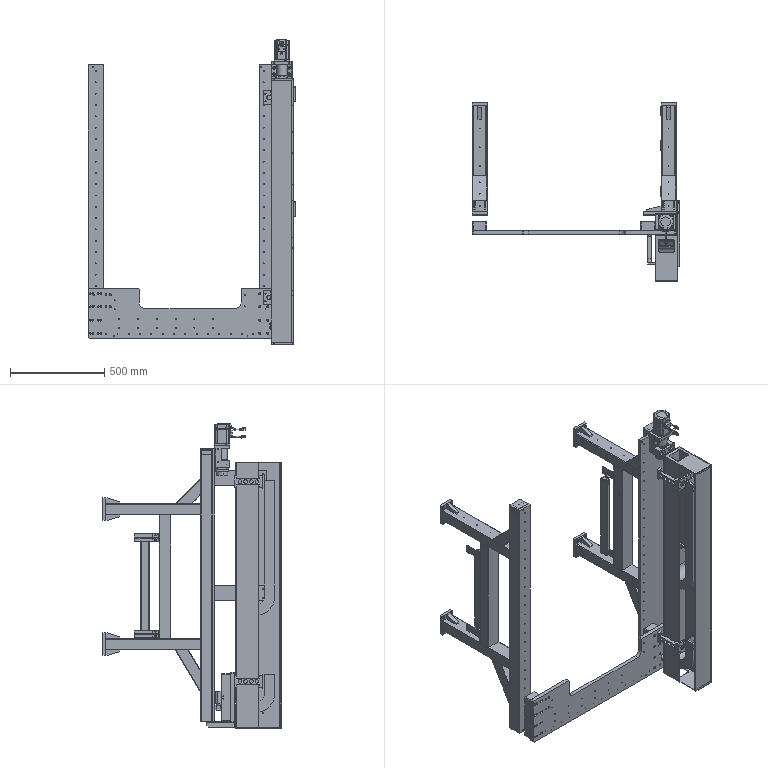Part | NX | 91 solids | 2923 faces | box 1102 x 947.5 x 1613 mm | volume 32221262 mm3 | plane 1561 | cylinder 1148 | cone 177 | spline 37 | commonest cylinder face diameters 5 x222 4.2 x124 5.236 x96 10 x67 3.3 x52 11 x45